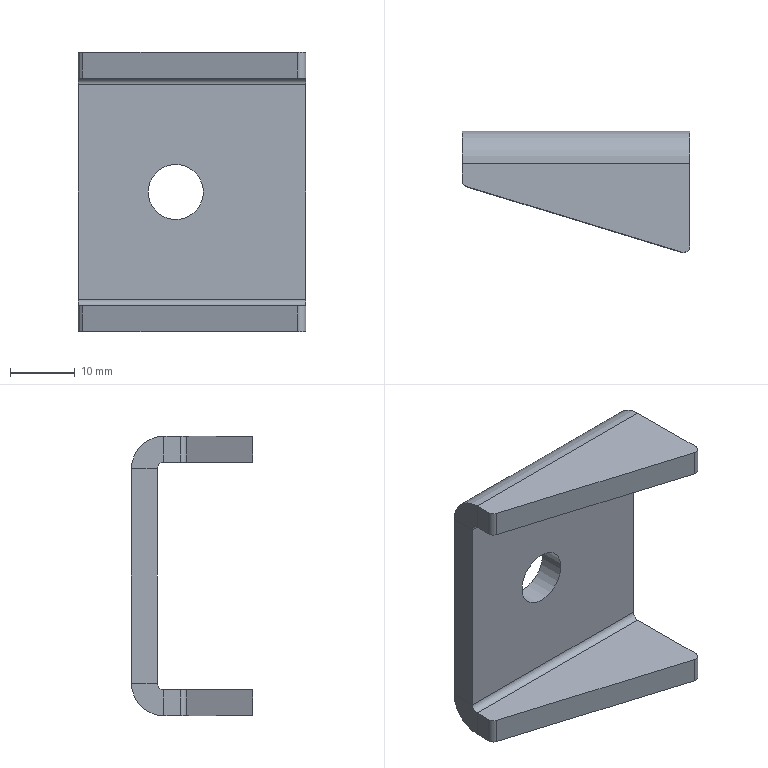Part | STEP file | 7100520 | 1 solid | 27 faces | box 35 x 18.649 x 43 mm | volume 8130 mm3 | plane 18 | cylinder 9 | commonest cylinder face diameters 2 x6 10 x2 8.5 x1